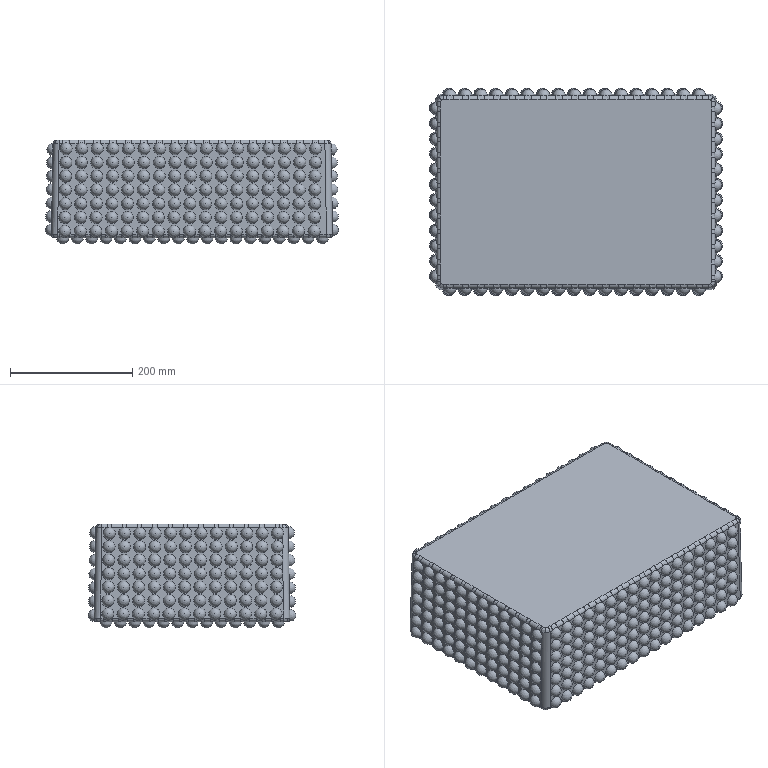Part | STEP file | CHERRIES_TO_CRATE1V11 | 1 solid | 927 faces | box 479.554 x 339.624 x 170 mm | volume 24539248 mm3 | sphere 659 | spline 132 | cylinder 128 | plane 8 | commonest cylinder face diameters 12 x124 20 x4